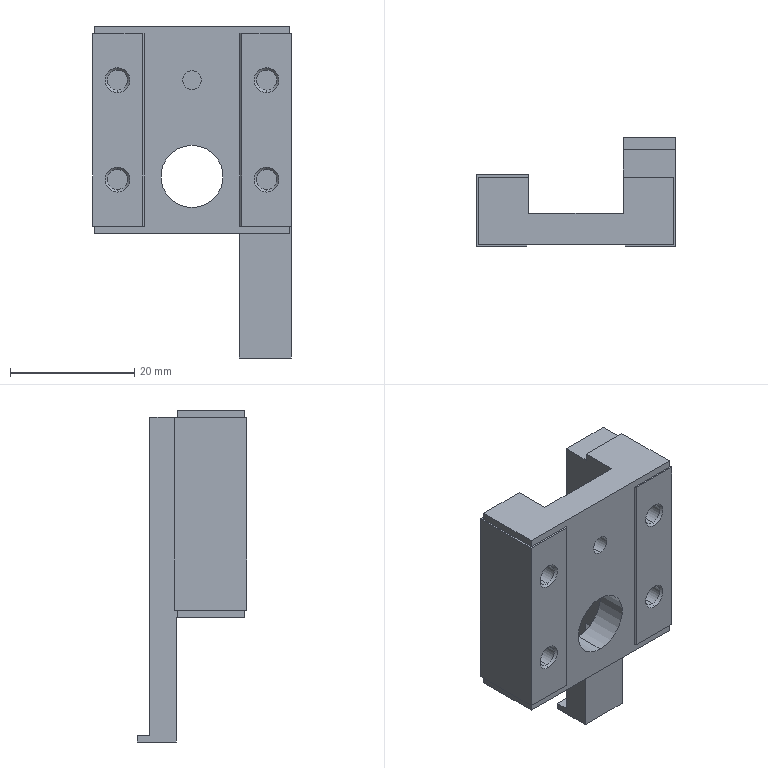Part | SolidWorks | features BaseBody 1 | 1 solid | 54 faces | box 32 x 17.6 x 53.4 mm | volume 10272 mm3 | plane 34 | cylinder 12 | cone 8 | commonest cylinder face diameters 3.242 x8 3 x2 10 x2
STEP:
#1=CARTESIAN_POINT('',(12.,0.379,7.079));
#2=VERTEX_POINT('',#1);
#3=CARTESIAN_POINT('',(12.,0.379,10.321));
#4=VERTEX_POINT('',#3);
#5=CARTESIAN_POINT('',(12.,0.379,8.7));
#6=DIRECTION('',(0.,-1.,0.));
#7=DIRECTION('',(0.,0.,-1.));
#8=AXIS2_PLACEMENT_3D('',#5,#6,#7);
#9=CIRCLE('',#8,1.621);
#10=EDGE_CURVE('',#2,#4,#9,.T.);
#11=ORIENTED_EDGE('',*,*,#10,.T.);
#12=CARTESIAN_POINT('',(12.,4.,10.321));
#13=VERTEX_POINT('',#12);
#14=CARTESIAN_POINT('',(12.,0.,10.321));
#15=DIRECTION('',(0.,1.,0.));
#16=VECTOR('',#15,1000.);
#17=LINE('',#14,#16);
#18=EDGE_CURVE('',#4,#13,#17,.T.);
#19=ORIENTED_EDGE('',*,*,#18,.T.);
#20=CARTESIAN_POINT('',(12.,4.,7.079));
#21=VERTEX_POINT('',#20);
#22=CARTESIAN_POINT('',(12.,4.,8.7));
#23=DIRECTION('',(0.,-1.,0.));
#24=DIRECTION('',(0.,0.,-1.));
#25=AXIS2_PLACEMENT_3D('',#22,#23,#24);
#26=CIRCLE('',#25,1.621);
#27=EDGE_CURVE('',#21,#13,#26,.T.);
#28=ORIENTED_EDGE('',*,*,#27,.F.);
#29=CARTESIAN_POINT('',(12.,0.,7.079));
#30=DIRECTION('',(0.,1.,0.));
#31=VECTOR('',#30,1000.);
#32=LINE('',#29,#31);
#33=EDGE_CURVE('',#2,#21,#32,.T.);
#34=ORIENTED_EDGE('',*,*,#33,.F.);
#35=EDGE_LOOP('',(#11,#19,#28,#34));
#36=FACE_OUTER_BOUND('',#35,.T.);
#37=CARTESIAN_POINT('',(12.,0.,8.7));
#38=DIRECTION('',(0.,1.,0.));
#39=DIRECTION('',(0.,0.,-1.));
#40=AXIS2_PLACEMENT_3D('',#37,#38,#39);
#41=CYLINDRICAL_SURFACE('',#40,1.621);
#42=ADVANCED_FACE('',(#36),#41,.F.);
#43=CARTESIAN_POINT('',(12.,0.379,8.7));
#44=DIRECTION('',(0.,-1.,0.));
#45=DIRECTION('',(0.,0.,-1.));
#46=AXIS2_PLACEMENT_3D('',#43,#44,#45);
#47=CIRCLE('',#46,1.621);
#48=EDGE_CURVE('',#4,#2,#47,.T.);
#49=ORIENTED_EDGE('',*,*,#48,.F.);
#50=CARTESIAN_POINT('',(12.,0.,10.7));
#51=VERTEX_POINT('',#50);
#52=CARTESIAN_POINT('',(12.,0.379,10.321));
#53=DIRECTION('',(0.,-0.7071,0.7071));
#54=VECTOR('',#53,1000.);
#55=LINE('',#52,#54);
#56=EDGE_CURVE('',#4,#51,#55,.T.);
#57=ORIENTED_EDGE('',*,*,#56,.T.);
#58=CARTESIAN_POINT('',(12.,0.,6.7));
#59=VERTEX_POINT('',#58);
#60=CARTESIAN_POINT('',(12.,0.,8.7));
#61=DIRECTION('',(0.,-1.,0.));
#62=DIRECTION('',(0.,0.,-1.));
#63=AXIS2_PLACEMENT_3D('',#60,#61,#62);
#64=CIRCLE('',#63,2.);
#65=EDGE_CURVE('',#51,#59,#64,.T.);
#66=ORIENTED_EDGE('',*,*,#65,.T.);
#67=CARTESIAN_POINT('',(12.,0.379,7.079));
#68=DIRECTION('',(0.,-0.7071,-0.7071));
#69=VECTOR('',#68,1000.);
#70=LINE('',#67,#69);
#71=EDGE_CURVE('',#2,#59,#70,.T.);
#72=ORIENTED_EDGE('',*,*,#71,.F.);
#73=EDGE_LOOP('',(#49,#57,#66,#72));
#74=FACE_OUTER_BOUND('',#73,.T.);
#75=CARTESIAN_POINT('',(12.,0.379,8.7));
#76=DIRECTION('',(0.,-1.,0.));
#77=DIRECTION('',(0.,0.,-1.));
#78=AXIS2_PLACEMENT_3D('',#75,#76,#77);
#79=CONICAL_SURFACE('',#78,1.621,0.7854);
#80=ADVANCED_FACE('',(#74),#79,.F.);
#81=CARTESIAN_POINT('',(-12.,0.379,7.079));
#82=VERTEX_POINT('',#81);
#83=CARTESIAN_POINT('',(-12.,0.379,10.321));
#84=VERTEX_POINT('',#83);
#85=CARTESIAN_POINT('',(-12.,0.379,8.7));
#86=DIRECTION('',(0.,-1.,0.));
#87=DIRECTION('',(0.,0.,-1.));
#88=AXIS2_PLACEMENT_3D('',#85,#86,#87);
#89=CIRCLE('',#88,1.621);
#90=EDGE_CURVE('',#82,#84,#89,.T.);
#91=ORIENTED_EDGE('',*,*,#90,.T.);
#92=CARTESIAN_POINT('',(-12.,4.,10.321));
#93=VERTEX_POINT('',#92);
#94=CARTESIAN_POINT('',(-12.,0.,10.321));
#95=DIRECTION('',(0.,1.,0.));
#96=VECTOR('',#95,1000.);
#97=LINE('',#94,#96);
#98=EDGE_CURVE('',#84,#93,#97,.T.);
#99=ORIENTED_EDGE('',*,*,#98,.T.);
#100=CARTESIAN_POINT('',(-12.,4.,7.079));
#101=VERTEX_POINT('',#100);
#102=CARTESIAN_POINT('',(-12.,4.,8.7));
#103=DIRECTION('',(0.,-1.,0.));
#104=DIRECTION('',(0.,0.,-1.));
#105=AXIS2_PLACEMENT_3D('',#102,#103,#104);
#106=CIRCLE('',#105,1.621);
#107=EDGE_CURVE('',#101,#93,#106,.T.);
#108=ORIENTED_EDGE('',*,*,#107,.F.);
#109=CARTESIAN_POINT('',(-12.,0.,7.079));
#110=DIRECTION('',(0.,1.,0.));
#111=VECTOR('',#110,1000.);
#112=LINE('',#109,#111);
#113=EDGE_CURVE('',#82,#101,#112,.T.);
#114=ORIENTED_EDGE('',*,*,#113,.F.);
#115=EDGE_LOOP('',(#91,#99,#108,#114));
#116=FACE_OUTER_BOUND('',#115,.T.);
#117=CARTESIAN_POINT('',(-12.,0.,8.7));
#118=DIRECTION('',(0.,1.,0.));
#119=DIRECTION('',(0.,0.,-1.));
#120=AXIS2_PLACEMENT_3D('',#117,#118,#119);
#121=CYLINDRICAL_SURFACE('',#120,1.621);
#122=ADVANCED_FACE('',(#116),#121,.F.);
#123=CARTESIAN_POINT('',(-12.,0.379,8.7));
#124=DIRECTION('',(0.,-1.,0.));
#125=DIRECTION('',(0.,0.,-1.));
#126=AXIS2_PLACEMENT_3D('',#123,#124,#125);
#127=CIRCLE('',#126,1.621);
#128=EDGE_CURVE('',#84,#82,#127,.T.);
#129=ORIENTED_EDGE('',*,*,#128,.F.);
#130=CARTESIAN_POINT('',(-12.,0.,10.7));
#131=VERTEX_POINT('',#130);
#132=CARTESIAN_POINT('',(-12.,0.379,10.321));
#133=DIRECTION('',(0.,-0.7071,0.7071));
#134=VECTOR('',#133,1000.);
#135=LINE('',#132,#134);
#136=EDGE_CURVE('',#84,#131,#135,.T.);
#137=ORIENTED_EDGE('',*,*,#136,.T.);
#138=CARTESIAN_POINT('',(-12.,0.,6.7));
#139=VERTEX_POINT('',#138);
#140=CARTESIAN_POINT('',(-12.,0.,8.7));
#141=DIRECTION('',(0.,-1.,0.));
#142=DIRECTION('',(0.,0.,-1.));
#143=AXIS2_PLACEMENT_3D('',#140,#141,#142);
#144=CIRCLE('',#143,2.);
#145=EDGE_CURVE('',#131,#139,#144,.T.);
#146=ORIENTED_EDGE('',*,*,#145,.T.);
#147=CARTESIAN_POINT('',(-12.,0.379,7.079));
#148=DIRECTION('',(0.,-0.7071,-0.7071));
#149=VECTOR('',#148,1000.);
#150=LINE('',#147,#149);
#151=EDGE_CURVE('',#82,#139,#150,.T.);
#152=ORIENTED_EDGE('',*,*,#151,.F.);
#153=EDGE_LOOP('',(#129,#137,#146,#152));
#154=FACE_OUTER_BOUND('',#153,.T.);
#155=CARTESIAN_POINT('',(-12.,0.379,8.7));
#156=DIRECTION('',(0.,-1.,0.));
#157=DIRECTION('',(0.,0.,-1.));
#158=AXIS2_PLACEMENT_3D('',#155,#156,#157);
#159=CONICAL_SURFACE('',#158,1.621,0.7854);
#160=ADVANCED_FACE('',(#154),#159,.F.);
#161=CARTESIAN_POINT('',(12.,0.379,23.079));
#162=VERTEX_POINT('',#161);
#163=CARTESIAN_POINT('',(12.,0.379,26.321));
#164=VERTEX_POINT('',#163);
#165=CARTESIAN_POINT('',(12.,0.379,24.7));
#166=DIRECTION('',(0.,-1.,0.));
#167=DIRECTION('',(0.,0.,-1.));
#168=AXIS2_PLACEMENT_3D('',#165,#166,#167);
#169=CIRCLE('',#168,1.621);
#170=EDGE_CURVE('',#162,#164,#169,.T.);
#171=ORIENTED_EDGE('',*,*,#170,.T.);
#172=CARTESIAN_POINT('',(12.,4.,26.321));
#173=VERTEX_POINT('',#172);
#174=CARTESIAN_POINT('',(12.,0.,26.321));
#175=DIRECTION('',(0.,1.,0.));
#176=VECTOR('',#175,1000.);
#177=LINE('',#174,#176);
#178=EDGE_CURVE('',#164,#173,#177,.T.);
#179=ORIENTED_EDGE('',*,*,#178,.T.);
#180=CARTESIAN_POINT('',(12.,4.,23.079));
#181=VERTEX_POINT('',#180);
#182=CARTESIAN_POINT('',(12.,4.,24.7));
#183=DIRECTION('',(0.,-1.,0.));
#184=DIRECTION('',(0.,0.,-1.));
#185=AXIS2_PLACEMENT_3D('',#182,#183,#184);
#186=CIRCLE('',#185,1.621);
#187=EDGE_CURVE('',#181,#173,#186,.T.);
#188=ORIENTED_EDGE('',*,*,#187,.F.);
#189=CARTESIAN_POINT('',(12.,0.,23.079));
#190=DIRECTION('',(0.,1.,0.));
#191=VECTOR('',#190,1000.);
#192=LINE('',#189,#191);
#193=EDGE_CURVE('',#162,#181,#192,.T.);
#194=ORIENTED_EDGE('',*,*,#193,.F.);
#195=EDGE_LOOP('',(#171,#179,#188,#194));
#196=FACE_OUTER_BOUND('',#195,.T.);
#197=CARTESIAN_POINT('',(12.,0.,24.7));
#198=DIRECTION('',(0.,1.,0.));
#199=DIRECTION('',(0.,0.,-1.));
#200=AXIS2_PLACEMENT_3D('',#197,#198,#199);
#201=CYLINDRICAL_SURFACE('',#200,1.621);
#202=ADVANCED_FACE('',(#196),#201,.F.);
#203=CARTESIAN_POINT('',(12.,0.379,24.7));
#204=DIRECTION('',(0.,-1.,0.));
#205=DIRECTION('',(0.,0.,-1.));
#206=AXIS2_PLACEMENT_3D('',#203,#204,#205);
#207=CIRCLE('',#206,1.621);
#208=EDGE_CURVE('',#164,#162,#207,.T.);
#209=ORIENTED_EDGE('',*,*,#208,.F.);
#210=CARTESIAN_POINT('',(12.,0.,26.7));
#211=VERTEX_POINT('',#210);
#212=CARTESIAN_POINT('',(12.,0.379,26.321));
#213=DIRECTION('',(0.,-0.7071,0.7071));
#214=VECTOR('',#213,1000.);
#215=LINE('',#212,#214);
#216=EDGE_CURVE('',#164,#211,#215,.T.);
#217=ORIENTED_EDGE('',*,*,#216,.T.);
#218=CARTESIAN_POINT('',(12.,0.,22.7));
#219=VERTEX_POINT('',#218);
#220=CARTESIAN_POINT('',(12.,0.,24.7));
#221=DIRECTION('',(0.,-1.,0.));
#222=DIRECTION('',(0.,0.,-1.));
#223=AXIS2_PLACEMENT_3D('',#220,#221,#222);
#224=CIRCLE('',#223,2.);
#225=EDGE_CURVE('',#211,#219,#224,.T.);
#226=ORIENTED_EDGE('',*,*,#225,.T.);
#227=CARTESIAN_POINT('',(12.,0.379,23.079));
#228=DIRECTION('',(0.,-0.7071,-0.7071));
#229=VECTOR('',#228,1000.);
#230=LINE('',#227,#229);
#231=EDGE_CURVE('',#162,#219,#230,.T.);
#232=ORIENTED_EDGE('',*,*,#231,.F.);
#233=EDGE_LOOP('',(#209,#217,#226,#232));
#234=FACE_OUTER_BOUND('',#233,.T.);
#235=CARTESIAN_POINT('',(12.,0.379,24.7));
#236=DIRECTION('',(0.,-1.,0.));
#237=DIRECTION('',(0.,0.,-1.));
#238=AXIS2_PLACEMENT_3D('',#235,#236,#237);
#239=CONICAL_SURFACE('',#238,1.621,0.7854);
#240=ADVANCED_FACE('',(#234),#239,.F.);
#241=CARTESIAN_POINT('',(-12.,0.379,23.079));
#242=VERTEX_POINT('',#241);
#243=CARTESIAN_POINT('',(-12.,0.379,26.321));
#244=VERTEX_POINT('',#243);
#245=CARTESIAN_POINT('',(-12.,0.379,24.7));
#246=DIRECTION('',(0.,-1.,0.));
#247=DIRECTION('',(0.,0.,-1.));
#248=AXIS2_PLACEMENT_3D('',#245,#246,#247);
#249=CIRCLE('',#248,1.621);
#250=EDGE_CURVE('',#242,#244,#249,.T.);
#251=ORIENTED_EDGE('',*,*,#250,.T.);
#252=CARTESIAN_POINT('',(-12.,4.,26.321));
#253=VERTEX_POINT('',#252);
#254=CARTESIAN_POINT('',(-12.,0.,26.321));
#255=DIRECTION('',(0.,1.,0.));
#256=VECTOR('',#255,1000.);
#257=LINE('',#254,#256);
#258=EDGE_CURVE('',#244,#253,#257,.T.);
#259=ORIENTED_EDGE('',*,*,#258,.T.);
#260=CARTESIAN_POINT('',(-12.,4.,23.079));
#261=VERTEX_POINT('',#260);
#262=CARTESIAN_POINT('',(-12.,4.,24.7));
#263=DIRECTION('',(0.,-1.,0.));
#264=DIRECTION('',(0.,0.,-1.));
#265=AXIS2_PLACEMENT_3D('',#262,#263,#264);
#266=CIRCLE('',#265,1.621);
#267=EDGE_CURVE('',#261,#253,#266,.T.);
#268=ORIENTED_EDGE('',*,*,#267,.F.);
#269=CARTESIAN_POINT('',(-12.,0.,23.079));
#270=DIRECTION('',(0.,1.,0.));
#271=VECTOR('',#270,1000.);
#272=LINE('',#269,#271);
#273=EDGE_CURVE('',#242,#261,#272,.T.);
#274=ORIENTED_EDGE('',*,*,#273,.F.);
#275=EDGE_LOOP('',(#251,#259,#268,#274));
#276=FACE_OUTER_BOUND('',#275,.T.);
#277=CARTESIAN_POINT('',(-12.,0.,24.7));
#278=DIRECTION('',(0.,1.,0.));
#279=DIRECTION('',(0.,0.,-1.));
#280=AXIS2_PLACEMENT_3D('',#277,#278,#279);
#281=CYLINDRICAL_SURFACE('',#280,1.621);
#282=ADVANCED_FACE('',(#276),#281,.F.);
#283=CARTESIAN_POINT('',(-12.,0.379,24.7));
#284=DIRECTION('',(0.,-1.,0.));
#285=DIRECTION('',(0.,0.,-1.));
#286=AXIS2_PLACEMENT_3D('',#283,#284,#285);
#287=CIRCLE('',#286,1.621);
#288=EDGE_CURVE('',#244,#242,#287,.T.);
#289=ORIENTED_EDGE('',*,*,#288,.F.);
#290=CARTESIAN_POINT('',(-12.,0.,26.7));
#291=VERTEX_POINT('',#290);
#292=CARTESIAN_POINT('',(-12.,0.379,26.321));
#293=DIRECTION('',(0.,-0.7071,0.7071));
#294=VECTOR('',#293,1000.);
#295=LINE('',#292,#294);
#296=EDGE_CURVE('',#244,#291,#295,.T.);
#297=ORIENTED_EDGE('',*,*,#296,.T.);
#298=CARTESIAN_POINT('',(-12.,0.,22.7));
#299=VERTEX_POINT('',#298);
#300=CARTESIAN_POINT('',(-12.,0.,24.7));
#301=DIRECTION('',(0.,-1.,0.));
#302=DIRECTION('',(0.,0.,-1.));
#303=AXIS2_PLACEMENT_3D('',#300,#301,#302);
#304=CIRCLE('',#303,2.);
#305=EDGE_CURVE('',#291,#299,#304,.T.);
#306=ORIENTED_EDGE('',*,*,#305,.T.);
#307=CARTESIAN_POINT('',(-12.,0.379,23.079));
#308=DIRECTION('',(0.,-0.7071,-0.7071));
#309=VECTOR('',#308,1000.);
#310=LINE('',#307,#309);
#311=EDGE_CURVE('',#242,#299,#310,.T.);
#312=ORIENTED_EDGE('',*,*,#311,.F.);
#313=EDGE_LOOP('',(#289,#297,#306,#312));
#314=FACE_OUTER_BOUND('',#313,.T.);
#315=CARTESIAN_POINT('',(-12.,0.379,24.7));
#316=DIRECTION('',(0.,-1.,0.));
#317=DIRECTION('',(0.,0.,-1.));
#318=AXIS2_PLACEMENT_3D('',#315,#316,#317);
#319=CONICAL_SURFACE('',#318,1.621,0.7854);
#320=ADVANCED_FACE('',(#314),#319,.F.);
#321=CARTESIAN_POINT('',(0.,0.3,23.2));
#322=VERTEX_POINT('',#321);
#323=CARTESIAN_POINT('',(0.,0.3,26.2));
#324=VERTEX_POINT('',#323);
#325=CARTESIAN_POINT('',(0.,0.3,24.7));
#326=DIRECTION('',(0.,-1.,0.));
#327=DIRECTION('',(0.,0.,1.));
#328=AXIS2_PLACEMENT_3D('',#325,#326,#327);
#329=CIRCLE('',#328,1.5);
#330=EDGE_CURVE('',#322,#324,#329,.T.);
#331=ORIENTED_EDGE('',*,*,#330,.T.);
#332=CARTESIAN_POINT('',(0.,3.3,26.2));
#333=VERTEX_POINT('',#332);
#334=CARTESIAN_POINT('',(0.,3.3,26.2));
#335=DIRECTION('',(0.,1.,0.));
#336=VECTOR('',#335,1000.);
#337=LINE('',#334,#336);
#338=EDGE_CURVE('',#324,#333,#337,.T.);
#339=ORIENTED_EDGE('',*,*,#338,.T.);
#340=CARTESIAN_POINT('',(0.,3.3,23.2));
#341=VERTEX_POINT('',#340);
#342=CARTESIAN_POINT('',(0.,3.3,24.7));
#343=DIRECTION('',(0.,1.,0.));
#344=DIRECTION('',(1.,0.,0.));
#345=AXIS2_PLACEMENT_3D('',#342,#343,#344);
#346=CIRCLE('',#345,1.5);
#347=EDGE_CURVE('',#333,#341,#346,.T.);
#348=ORIENTED_EDGE('',*,*,#347,.T.);
#349=CARTESIAN_POINT('',(0.,3.3,23.2));
#350=DIRECTION('',(0.,1.,0.));
#351=VECTOR('',#350,1000.);
#352=LINE('',#349,#351);
#353=EDGE_CURVE('',#322,#341,#352,.T.);
#354=ORIENTED_EDGE('',*,*,#353,.F.);
#355=EDGE_LOOP('',(#331,#339,#348,#354));
#356=FACE_OUTER_BOUND('',#355,.T.);
#357=CARTESIAN_POINT('',(0.,3.3,24.7));
#358=DIRECTION('',(0.,1.,0.));
#359=DIRECTION('',(0.,0.,-1.));
#360=AXIS2_PLACEMENT_3D('',#357,#358,#359);
#361=CYLINDRICAL_SURFACE('',#360,1.5);
#362=ADVANCED_FACE('',(#356),#361,.F.);
#363=CARTESIAN_POINT('',(0.,0.3,4.2));
#364=VERTEX_POINT('',#363);
#365=CARTESIAN_POINT('',(0.,0.3,14.2));
#366=VERTEX_POINT('',#365);
#367=CARTESIAN_POINT('',(0.,0.3,9.2));
#368=DIRECTION('',(0.,-1.,0.));
#369=DIRECTION('',(0.,0.,1.));
#370=AXIS2_PLACEMENT_3D('',#367,#368,#369);
#371=CIRCLE('',#370,5.);
#372=EDGE_CURVE('',#364,#366,#371,.T.);
#373=ORIENTED_EDGE('',*,*,#372,.T.);
#374=CARTESIAN_POINT('',(0.,5.3,14.2));
#375=VERTEX_POINT('',#374);
#376=CARTESIAN_POINT('',(0.,5.5,14.2));
#377=DIRECTION('',(0.,1.,0.));
#378=VECTOR('',#377,1000.);
#379=LINE('',#376,#378);
#380=EDGE_CURVE('',#366,#375,#379,.T.);
#381=ORIENTED_EDGE('',*,*,#380,.T.);
#382=CARTESIAN_POINT('',(0.,5.3,4.2));
#383=VERTEX_POINT('',#382);
#384=CARTESIAN_POINT('',(0.,5.3,9.2));
#385=DIRECTION('',(0.,1.,0.));
#386=DIRECTION('',(0.,0.,-1.));
#387=AXIS2_PLACEMENT_3D('',#384,#385,#386);
#388=CIRCLE('',#387,5.);
#389=EDGE_CURVE('',#375,#383,#388,.T.);
#390=ORIENTED_EDGE('',*,*,#389,.T.);
#391=CARTESIAN_POINT('',(0.,5.5,4.2));
#392=DIRECTION('',(0.,1.,0.));
#393=VECTOR('',#392,1000.);
#394=LINE('',#391,#393);
#395=EDGE_CURVE('',#364,#383,#394,.T.);
#396=ORIENTED_EDGE('',*,*,#395,.F.);
#397=EDGE_LOOP('',(#373,#381,#390,#396));
#398=FACE_OUTER_BOUND('',#397,.T.);
#399=CARTESIAN_POINT('',(0.,5.5,9.2));
#400=DIRECTION('',(0.,1.,0.));
#401=DIRECTION('',(0.,0.,-1.));
#402=AXIS2_PLACEMENT_3D('',#399,#400,#401);
#403=CYLINDRICAL_SURFACE('',#402,5.);
#404=ADVANCED_FACE('',(#398),#403,.F.);
#405=CARTESIAN_POINT('',(15.7,11.3,1.2));
#406=VERTEX_POINT('',#405);
#407=CARTESIAN_POINT('',(15.7,0.3,1.2));
#408=VERTEX_POINT('',#407);
#409=CARTESIAN_POINT('',(15.7,11.6,1.2));
#410=DIRECTION('',(0.,-1.,0.));
#411=VECTOR('',#410,1000.);
#412=LINE('',#409,#411);
#413=EDGE_CURVE('',#406,#408,#412,.T.);
#414=ORIENTED_EDGE('',*,*,#413,.F.);
#415=CARTESIAN_POINT('',(16.,11.3,1.2));
#416=VERTEX_POINT('',#415);
#417=CARTESIAN_POINT('',(7.6,11.3,1.2));
#418=DIRECTION('',(1.,0.,0.));
#419=VECTOR('',#418,1000.);
#420=LINE('',#417,#419);
#421=EDGE_CURVE('',#406,#416,#420,.T.);
#422=ORIENTED_EDGE('',*,*,#421,.T.);
#423=CARTESIAN_POINT('',(16.,0.,1.2));
#424=VERTEX_POINT('',#423);
#425=CARTESIAN_POINT('',(16.,0.,1.2));
#426=DIRECTION('',(0.,1.,0.));
#427=VECTOR('',#426,1000.);
#428=LINE('',#425,#427);
#429=EDGE_CURVE('',#424,#416,#428,.T.);
#430=ORIENTED_EDGE('',*,*,#429,.F.);
#431=CARTESIAN_POINT('',(8.,0.,1.2));
#432=VERTEX_POINT('',#431);
#433=CARTESIAN_POINT('',(-16.,0.,1.2));
#434=DIRECTION('',(1.,0.,0.));
#435=VECTOR('',#434,1000.);
#436=LINE('',#433,#435);
#437=EDGE_CURVE('',#432,#424,#436,.T.);
#438=ORIENTED_EDGE('',*,*,#437,.F.);
#439=CARTESIAN_POINT('',(7.7,0.3,1.2));
#440=VERTEX_POINT('',#439);
#441=CARTESIAN_POINT('',(7.7,0.3,1.2));
#442=DIRECTION('',(0.7071,-0.7071,0.));
#443=VECTOR('',#442,1000.);
#444=LINE('',#441,#443);
#445=EDGE_CURVE('',#440,#432,#444,.T.);
#446=ORIENTED_EDGE('',*,*,#445,.F.);
#447=CARTESIAN_POINT('',(15.7,0.3,1.2));
#448=DIRECTION('',(-1.,0.,0.));
#449=VECTOR('',#448,1000.);
#450=LINE('',#447,#449);
#451=EDGE_CURVE('',#408,#440,#450,.T.);
#452=ORIENTED_EDGE('',*,*,#451,.F.);
#453=EDGE_LOOP('',(#414,#422,#430,#438,#446,#452));
#454=FACE_OUTER_BOUND('',#453,.T.);
#455=CARTESIAN_POINT('',(0.,0.,1.2));
#456=DIRECTION('',(0.,0.,1.));
#457=DIRECTION('',(1.,0.,0.));
#458=AXIS2_PLACEMENT_3D('',#455,#456,#457);
#459=PLANE('',#458);
#460=ADVANCED_FACE('',(#454),#459,.F.);
#461=CARTESIAN_POINT('',(7.7,0.3,32.2));
#462=VERTEX_POINT('',#461);
#463=CARTESIAN_POINT('',(8.,0.,32.2));
#464=VERTEX_POINT('',#463);
#465=CARTESIAN_POINT('',(7.7,0.3,32.2));
#466=DIRECTION('',(0.7071,-0.7071,0.));
#467=VECTOR('',#466,1000.);
#468=LINE('',#465,#467);
#469=EDGE_CURVE('',#462,#464,#468,.T.);
#470=ORIENTED_EDGE('',*,*,#469,.T.);
#471=CARTESIAN_POINT('',(16.,0.,32.2));
#472=VERTEX_POINT('',#471);
#473=CARTESIAN_POINT('',(-16.,0.,32.2));
#474=DIRECTION('',(1.,0.,0.));
#475=VECTOR('',#474,1000.);
#476=LINE('',#473,#475);
#477=EDGE_CURVE('',#464,#472,#476,.T.);
#478=ORIENTED_EDGE('',*,*,#477,.T.);
#479=CARTESIAN_POINT('',(16.,15.6,32.2));
#480=VERTEX_POINT('',#479);
#481=CARTESIAN_POINT('',(16.,0.,32.2));
#482=DIRECTION('',(0.,1.,0.));
#483=VECTOR('',#482,1000.);
#484=LINE('',#481,#483);
#485=EDGE_CURVE('',#472,#480,#484,.T.);
#486=ORIENTED_EDGE('',*,*,#485,.T.);
#487=CARTESIAN_POINT('',(7.6,15.6,32.2));
#488=VERTEX_POINT('',#487);
#489=CARTESIAN_POINT('',(16.,15.6,32.2));
#490=DIRECTION('',(-1.,0.,0.));
#491=VECTOR('',#490,1000.);
#492=LINE('',#489,#491);
#493=EDGE_CURVE('',#480,#488,#492,.T.);
#494=ORIENTED_EDGE('',*,*,#493,.T.);
#495=CARTESIAN_POINT('',(7.6,11.1,32.2));
#496=VERTEX_POINT('',#495);
#497=CARTESIAN_POINT('',(7.6,15.6,32.2));
#498=DIRECTION('',(0.,-1.,0.));
#499=VECTOR('',#498,1000.);
#500=LINE('',#497,#499);
#501=EDGE_CURVE('',#488,#496,#500,.T.);
#502=ORIENTED_EDGE('',*,*,#501,.T.);
#503=CARTESIAN_POINT('',(15.7,11.1,32.2));
#504=VERTEX_POINT('',#503);
#505=CARTESIAN_POINT('',(7.6,11.1,32.2));
#506=DIRECTION('',(1.,0.,0.));
#507=VECTOR('',#506,1000.);
#508=LINE('',#505,#507);
#509=EDGE_CURVE('',#496,#504,#508,.T.);
#510=ORIENTED_EDGE('',*,*,#509,.T.);
#511=CARTESIAN_POINT('',(15.7,0.3,32.2));
#512=VERTEX_POINT('',#511);
#513=CARTESIAN_POINT('',(15.7,11.1,32.2));
#514=DIRECTION('',(0.,-1.,0.));
#515=VECTOR('',#514,1000.);
#516=LINE('',#513,#515);
#517=EDGE_CURVE('',#504,#512,#516,.T.);
#518=ORIENTED_EDGE('',*,*,#517,.T.);
#519=CARTESIAN_POINT('',(15.7,0.3,32.2));
#520=DIRECTION('',(-1.,0.,0.));
#521=VECTOR('',#520,1000.);
#522=LINE('',#519,#521);
#523=EDGE_CURVE('',#512,#462,#522,.T.);
#524=ORIENTED_EDGE('',*,*,#523,.T.);
#525=EDGE_LOOP('',(#470,#478,#486,#494,#502,#510,#518,#524));
#526=FACE_OUTER_BOUND('',#525,.T.);
#527=CARTESIAN_POINT('',(0.,0.,32.2));
#528=DIRECTION('',(0.,0.,1.));
#529=DIRECTION('',(1.,0.,0.));
#530=AXIS2_PLACEMENT_3D('',#527,#528,#529);
#531=PLANE('',#530);
#532=ADVANCED_FACE('',(#526),#531,.T.);
#533=CARTESIAN_POINT('',(16.,17.6,-19.));
#534=VERTEX_POINT('',#533);
#535=CARTESIAN_POINT('',(7.6,17.6,-19.));
#536=VERTEX_POINT('',#535);
#537=CARTESIAN_POINT('',(16.,17.6,-19.));
#538=DIRECTION('',(-1.,0.,0.));
#539=VECTOR('',#538,1000.);
#540=LINE('',#537,#539);
#541=EDGE_CURVE('',#534,#536,#540,.T.);
#542=ORIENTED_EDGE('',*,*,#541,.T.);
#543=CARTESIAN_POINT('',(7.6,15.6,-19.));
#544=VERTEX_POINT('',#543);
#545=CARTESIAN_POINT('',(7.6,17.6,-19.));
#546=DIRECTION('',(0.,-1.,0.));
#547=VECTOR('',#546,1000.);
#548=LINE('',#545,#547);
#549=EDGE_CURVE('',#536,#544,#548,.T.);
#550=ORIENTED_EDGE('',*,*,#549,.T.);
#551=CARTESIAN_POINT('',(16.,15.6,-19.));
#552=VERTEX_POINT('',#551);
#553=CARTESIAN_POINT('',(7.6,15.6,-19.));
#554=DIRECTION('',(1.,0.,0.));
#555=VECTOR('',#554,1000.);
#556=LINE('',#553,#555);
#557=EDGE_CURVE('',#544,#552,#556,.T.);
#558=ORIENTED_EDGE('',*,*,#557,.T.);
#559=CARTESIAN_POINT('',(16.,15.6,-19.));
#560=DIRECTION('',(0.,1.,0.));
#561=VECTOR('',#560,1000.);
#562=LINE('',#559,#561);
#563=EDGE_CURVE('',#552,#534,#562,.T.);
#564=ORIENTED_EDGE('',*,*,#563,.T.);
#565=EDGE_LOOP('',(#542,#550,#558,#564));
#566=FACE_OUTER_BOUND('',#565,.T.);
#567=CARTESIAN_POINT('',(0.,0.,-19.));
#568=DIRECTION('',(0.,0.,1.));
#569=DIRECTION('',(1.,0.,0.));
#570=AXIS2_PLACEMENT_3D('',#567,#568,#569);
#571=PLANE('',#570);
#572=ADVANCED_FACE('',(#566),#571,.T.);
#573=CARTESIAN_POINT('',(16.,17.6,-20.));
#574=VERTEX_POINT('',#573);
#575=CARTESIAN_POINT('',(7.6,17.6,-20.));
#576=VERTEX_POINT('',#575);
#577=CARTESIAN_POINT('',(16.,17.6,-20.));
#578=DIRECTION('',(-1.,0.,0.));
#579=VECTOR('',#578,1000.);
#580=LINE('',#577,#579);
#581=EDGE_CURVE('',#574,#576,#580,.T.);
#582=ORIENTED_EDGE('',*,*,#581,.T.);
#583=CARTESIAN_POINT('',(7.6,17.6,-19.));
#584=DIRECTION('',(0.,0.,-1.));
#585=VECTOR('',#584,1000.);
#586=LINE('',#583,#585);
#587=EDGE_CURVE('',#536,#576,#586,.T.);
#588=ORIENTED_EDGE('',*,*,#587,.F.);
#589=ORIENTED_EDGE('',*,*,#541,.F.);
#590=CARTESIAN_POINT('',(16.,17.6,-19.));
#591=DIRECTION('',(0.,0.,-1.));
#592=VECTOR('',#591,1000.);
#593=LINE('',#590,#592);
#594=EDGE_CURVE('',#534,#574,#593,.T.);
#595=ORIENTED_EDGE('',*,*,#594,.T.);
#596=EDGE_LOOP('',(#582,#588,#589,#595));
#597=FACE_OUTER_BOUND('',#596,.T.);
#598=CARTESIAN_POINT('',(16.,17.6,-19.));
#599=DIRECTION('',(0.,-1.,0.));
#600=DIRECTION('',(0.,0.,-1.));
#601=AXIS2_PLACEMENT_3D('',#598,#599,#600);
#602=PLANE('',#601);
#603=ADVANCED_FACE('',(#597),#602,.F.);
#604=ORIENTED_EDGE('',*,*,#380,.F.);
#605=CARTESIAN_POINT('',(0.,0.3,9.2));
#606=DIRECTION('',(0.,-1.,0.));
#607=DIRECTION('',(0.,0.,1.));
#608=AXIS2_PLACEMENT_3D('',#605,#606,#607);
#609=CIRCLE('',#608,5.);
#610=EDGE_CURVE('',#366,#364,#609,.T.);
#611=ORIENTED_EDGE('',*,*,#610,.T.);
#612=ORIENTED_EDGE('',*,*,#395,.T.);
#613=CARTESIAN_POINT('',(0.,5.3,9.2));
#614=DIRECTION('',(0.,1.,0.));
#615=DIRECTION('',(0.,0.,-1.));
#616=AXIS2_PLACEMENT_3D('',#613,#614,#615);
#617=CIRCLE('',#616,5.);
#618=EDGE_CURVE('',#383,#375,#617,.T.);
#619=ORIENTED_EDGE('',*,*,#618,.T.);
#620=EDGE_LOOP('',(#604,#611,#612,#619));
#621=FACE_OUTER_BOUND('',#620,.T.);
#622=CARTESIAN_POINT('',(0.,5.5,9.2));
#623=DIRECTION('',(0.,1.,0.));
#624=DIRECTION('',(0.,0.,-1.));
#625=AXIS2_PLACEMENT_3D('',#622,#623,#624);
#626=CYLINDRICAL_SURFACE('',#625,5.);
#627=ADVANCED_FACE('',(#621),#626,.F.);
#628=CARTESIAN_POINT('',(0.,3.3,24.7));
#629=DIRECTION('',(0.,1.,0.));
#630=DIRECTION('',(1.,0.,0.));
#631=AXIS2_PLACEMENT_3D('',#628,#629,#630);
#632=CIRCLE('',#631,1.5);
#633=EDGE_CURVE('',#341,#333,#632,.T.);
#634=ORIENTED_EDGE('',*,*,#633,.F.);
#635=ORIENTED_EDGE('',*,*,#347,.F.);
#636=EDGE_LOOP('',(#634,#635));
#637=FACE_OUTER_BOUND('',#636,.T.);
#638=CARTESIAN_POINT('',(0.,3.3,24.7));
#639=DIRECTION('',(0.,1.,0.));
#640=DIRECTION('',(1.,0.,0.));
#641=AXIS2_PLACEMENT_3D('',#638,#639,#640);
#642=PLANE('',#641);
#643=ADVANCED_FACE('',(#637),#642,.F.);
#644=ORIENTED_EDGE('',*,*,#338,.F.);
#645=CARTESIAN_POINT('',(0.,0.3,24.7));
#646=DIRECTION('',(0.,-1.,0.));
#647=DIRECTION('',(0.,0.,1.));
#648=AXIS2_PLACEMENT_3D('',#645,#646,#647);
#649=CIRCLE('',#648,1.5);
#650=EDGE_CURVE('',#324,#322,#649,.T.);
#651=ORIENTED_EDGE('',*,*,#650,.T.);
#652=ORIENTED_EDGE('',*,*,#353,.T.);
#653=ORIENTED_EDGE('',*,*,#633,.T.);
#654=EDGE_LOOP('',(#644,#651,#652,#653));
#655=FACE_OUTER_BOUND('',#654,.T.);
#656=CARTESIAN_POINT('',(0.,3.3,24.7));
#657=DIRECTION('',(0.,1.,0.));
#658=DIRECTION('',(0.,0.,-1.));
#659=AXIS2_PLACEMENT_3D('',#656,#657,#658);
#660=CYLINDRICAL_SURFACE('',#659,1.5);
#661=ADVANCED_FACE('',(#655),#660,.F.);
#662=ORIENTED_EDGE('',*,*,#296,.F.);
#663=ORIENTED_EDGE('',*,*,#250,.F.);
#664=ORIENTED_EDGE('',*,*,#311,.T.);
#665=CARTESIAN_POINT('',(-12.,0.,24.7));
#666=DIRECTION('',(0.,-1.,0.));
#667=DIRECTION('',(0.,0.,-1.));
#668=AXIS2_PLACEMENT_3D('',#665,#666,#667);
#669=CIRCLE('',#668,2.);
#670=EDGE_CURVE('',#299,#291,#669,.T.);
#671=ORIENTED_EDGE('',*,*,#670,.T.);
#672=EDGE_LOOP('',(#662,#663,#664,#671));
#673=FACE_OUTER_BOUND('',#672,.T.);
#674=CARTESIAN_POINT('',(-12.,0.379,24.7));
#675=DIRECTION('',(0.,-1.,0.));
#676=DIRECTION('',(0.,0.,-1.));
#677=AXIS2_PLACEMENT_3D('',#674,#675,#676);
#678=CONICAL_SURFACE('',#677,1.621,0.7854);
#679=ADVANCED_FACE('',(#673),#678,.F.);
#680=ORIENTED_EDGE('',*,*,#258,.F.);
#681=ORIENTED_EDGE('',*,*,#288,.T.);
#682=ORIENTED_EDGE('',*,*,#273,.T.);
#683=CARTESIAN_POINT('',(-12.,4.,24.7));
#684=DIRECTION('',(0.,-1.,0.));
#685=DIRECTION('',(0.,0.,-1.));
#686=AXIS2_PLACEMENT_3D('',#683,#684,#685);
#687=CIRCLE('',#686,1.621);
#688=EDGE_CURVE('',#253,#261,#687,.T.);
#689=ORIENTED_EDGE('',*,*,#688,.F.);
#690=EDGE_LOOP('',(#680,#681,#682,#689));
#691=FACE_OUTER_BOUND('',#690,.T.);
#692=CARTESIAN_POINT('',(-12.,0.,24.7));
#693=DIRECTION('',(0.,1.,0.));
#694=DIRECTION('',(0.,0.,-1.));
#695=AXIS2_PLACEMENT_3D('',#692,#693,#694);
#696=CYLINDRICAL_SURFACE('',#695,1.621);
#697=ADVANCED_FACE('',(#691),#696,.F.);
#698=ORIENTED_EDGE('',*,*,#267,.T.);
#699=ORIENTED_EDGE('',*,*,#688,.T.);
#700=EDGE_LOOP('',(#698,#699));
#701=FACE_OUTER_BOUND('',#700,.T.);
#702=CARTESIAN_POINT('',(-12.,4.,24.7));
#703=DIRECTION('',(0.,-1.,0.));
#704=DIRECTION('',(0.,0.,-1.));
#705=AXIS2_PLACEMENT_3D('',#702,#703,#704);
#706=PLANE('',#705);
#707=ADVANCED_FACE('',(#701),#706,.T.);
#708=ORIENTED_EDGE('',*,*,#216,.F.);
#709=ORIENTED_EDGE('',*,*,#170,.F.);
#710=ORIENTED_EDGE('',*,*,#231,.T.);
#711=CARTESIAN_POINT('',(12.,0.,24.7));
#712=DIRECTION('',(0.,-1.,0.));
#713=DIRECTION('',(0.,0.,-1.));
#714=AXIS2_PLACEMENT_3D('',#711,#712,#713);
#715=CIRCLE('',#714,2.);
#716=EDGE_CURVE('',#219,#211,#715,.T.);
#717=ORIENTED_EDGE('',*,*,#716,.T.);
#718=EDGE_LOOP('',(#708,#709,#710,#717));
#719=FACE_OUTER_BOUND('',#718,.T.);
#720=CARTESIAN_POINT('',(12.,0.379,24.7));
#721=DIRECTION('',(0.,-1.,0.));
#722=DIRECTION('',(0.,0.,-1.));
#723=AXIS2_PLACEMENT_3D('',#720,#721,#722);
#724=CONICAL_SURFACE('',#723,1.621,0.7854);
#725=ADVANCED_FACE('',(#719),#724,.F.);
#726=ORIENTED_EDGE('',*,*,#178,.F.);
#727=ORIENTED_EDGE('',*,*,#208,.T.);
#728=ORIENTED_EDGE('',*,*,#193,.T.);
#729=CARTESIAN_POINT('',(12.,4.,24.7));
#730=DIRECTION('',(0.,-1.,0.));
#731=DIRECTION('',(0.,0.,-1.));
#732=AXIS2_PLACEMENT_3D('',#729,#730,#731);
#733=CIRCLE('',#732,1.621);
#734=EDGE_CURVE('',#173,#181,#733,.T.);
#735=ORIENTED_EDGE('',*,*,#734,.F.);
#736=EDGE_LOOP('',(#726,#727,#728,#735));
#737=FACE_OUTER_BOUND('',#736,.T.);
#738=CARTESIAN_POINT('',(12.,0.,24.7));
#739=DIRECTION('',(0.,1.,0.));
#740=DIRECTION('',(0.,0.,-1.));
#741=AXIS2_PLACEMENT_3D('',#738,#739,#740);
#742=CYLINDRICAL_SURFACE('',#741,1.621);
#743=ADVANCED_FACE('',(#737),#742,.F.);
#744=ORIENTED_EDGE('',*,*,#187,.T.);
#745=ORIENTED_EDGE('',*,*,#734,.T.);
#746=EDGE_LOOP('',(#744,#745));
#747=FACE_OUTER_BOUND('',#746,.T.);
#748=CARTESIAN_POINT('',(12.,4.,24.7));
#749=DIRECTION('',(0.,-1.,0.));
#750=DIRECTION('',(0.,0.,-1.));
#751=AXIS2_PLACEMENT_3D('',#748,#749,#750);
#752=PLANE('',#751);
#753=ADVANCED_FACE('',(#747),#752,.T.);
#754=ORIENTED_EDGE('',*,*,#136,.F.);
#755=ORIENTED_EDGE('',*,*,#90,.F.);
#756=ORIENTED_EDGE('',*,*,#151,.T.);
#757=CARTESIAN_POINT('',(-12.,0.,8.7));
#758=DIRECTION('',(0.,-1.,0.));
#759=DIRECTION('',(0.,0.,-1.));
#760=AXIS2_PLACEMENT_3D('',#757,#758,#759);
#761=CIRCLE('',#760,2.);
#762=EDGE_CURVE('',#139,#131,#761,.T.);
#763=ORIENTED_EDGE('',*,*,#762,.T.);
#764=EDGE_LOOP('',(#754,#755,#756,#763));
#765=FACE_OUTER_BOUND('',#764,.T.);
#766=CARTESIAN_POINT('',(-12.,0.379,8.7));
#767=DIRECTION('',(0.,-1.,0.));
#768=DIRECTION('',(0.,0.,-1.));
#769=AXIS2_PLACEMENT_3D('',#766,#767,#768);
#770=CONICAL_SURFACE('',#769,1.621,0.7854);
#771=ADVANCED_FACE('',(#765),#770,.F.);
#772=ORIENTED_EDGE('',*,*,#98,.F.);
#773=ORIENTED_EDGE('',*,*,#128,.T.);
#774=ORIENTED_EDGE('',*,*,#113,.T.);
#775=CARTESIAN_POINT('',(-12.,4.,8.7));
#776=DIRECTION('',(0.,-1.,0.));
#777=DIRECTION('',(0.,0.,-1.));
#778=AXIS2_PLACEMENT_3D('',#775,#776,#777);
#779=CIRCLE('',#778,1.621);
#780=EDGE_CURVE('',#93,#101,#779,.T.);
#781=ORIENTED_EDGE('',*,*,#780,.F.);
#782=EDGE_LOOP('',(#772,#773,#774,#781));
#783=FACE_OUTER_BOUND('',#782,.T.);
#784=CARTESIAN_POINT('',(-12.,0.,8.7));
#785=DIRECTION('',(0.,1.,0.));
#786=DIRECTION('',(0.,0.,-1.));
#787=AXIS2_PLACEMENT_3D('',#784,#785,#786);
#788=CYLINDRICAL_SURFACE('',#787,1.621);
#789=ADVANCED_FACE('',(#783),#788,.F.);
#790=ORIENTED_EDGE('',*,*,#107,.T.);
#791=ORIENTED_EDGE('',*,*,#780,.T.);
#792=EDGE_LOOP('',(#790,#791));
#793=FACE_OUTER_BOUND('',#792,.T.);
#794=CARTESIAN_POINT('',(-12.,4.,8.7));
#795=DIRECTION('',(0.,-1.,0.));
#796=DIRECTION('',(0.,0.,-1.));
#797=AXIS2_PLACEMENT_3D('',#794,#795,#796);
#798=PLANE('',#797);
#799=ADVANCED_FACE('',(#793),#798,.T.);
#800=ORIENTED_EDGE('',*,*,#56,.F.);
#801=ORIENTED_EDGE('',*,*,#10,.F.);
#802=ORIENTED_EDGE('',*,*,#71,.T.);
#803=CARTESIAN_POINT('',(12.,0.,8.7));
#804=DIRECTION('',(0.,-1.,0.));
#805=DIRECTION('',(0.,0.,-1.));
#806=AXIS2_PLACEMENT_3D('',#803,#804,#805);
#807=CIRCLE('',#806,2.);
#808=EDGE_CURVE('',#59,#51,#807,.T.);
#809=ORIENTED_EDGE('',*,*,#808,.T.);
#810=EDGE_LOOP('',(#800,#801,#802,#809));
#811=FACE_OUTER_BOUND('',#810,.T.);
#812=CARTESIAN_POINT('',(12.,0.379,8.7));
#813=DIRECTION('',(0.,-1.,0.));
#814=DIRECTION('',(0.,0.,-1.));
#815=AXIS2_PLACEMENT_3D('',#812,#813,#814);
#816=CONICAL_SURFACE('',#815,1.621,0.7854);
#817=ADVANCED_FACE('',(#811),#816,.F.);
#818=ORIENTED_EDGE('',*,*,#18,.F.);
#819=ORIENTED_EDGE('',*,*,#48,.T.);
#820=ORIENTED_EDGE('',*,*,#33,.T.);
#821=CARTESIAN_POINT('',(12.,4.,8.7));
#822=DIRECTION('',(0.,-1.,0.));
#823=DIRECTION('',(0.,0.,-1.));
#824=AXIS2_PLACEMENT_3D('',#821,#822,#823);
#825=CIRCLE('',#824,1.621);
#826=EDGE_CURVE('',#13,#21,#825,.T.);
#827=ORIENTED_EDGE('',*,*,#826,.F.);
#828=EDGE_LOOP('',(#818,#819,#820,#827));
#829=FACE_OUTER_BOUND('',#828,.T.);
#830=CARTESIAN_POINT('',(12.,0.,8.7));
#831=DIRECTION('',(0.,1.,0.));
#832=DIRECTION('',(0.,0.,-1.));
#833=AXIS2_PLACEMENT_3D('',#830,#831,#832);
#834=CYLINDRICAL_SURFACE('',#833,1.621);
#835=ADVANCED_FACE('',(#829),#834,.F.);
#836=ORIENTED_EDGE('',*,*,#27,.T.);
#837=ORIENTED_EDGE('',*,*,#826,.T.);
#838=EDGE_LOOP('',(#836,#837));
#839=FACE_OUTER_BOUND('',#838,.T.);
#840=CARTESIAN_POINT('',(12.,4.,8.7));
#841=DIRECTION('',(0.,-1.,0.));
#842=DIRECTION('',(0.,0.,-1.));
#843=AXIS2_PLACEMENT_3D('',#840,#841,#842);
#844=PLANE('',#843);
#845=ADVANCED_FACE('',(#839),#844,.T.);
#846=CARTESIAN_POINT('',(7.6,11.3,-20.));
#847=VERTEX_POINT('',#846);
#848=CARTESIAN_POINT('',(7.6,15.6,-20.));
#849=DIRECTION('',(0.,-1.,0.));
#850=VECTOR('',#849,1000.);
#851=LINE('',#848,#850);
#852=EDGE_CURVE('',#576,#847,#851,.T.);
#853=ORIENTED_EDGE('',*,*,#852,.F.);
#854=ORIENTED_EDGE('',*,*,#581,.F.);
#855=CARTESIAN_POINT('',(16.,11.3,-20.));
#856=VERTEX_POINT('',#855);
#857=CARTESIAN_POINT('',(16.,11.3,-20.));
#858=DIRECTION('',(0.,1.,0.));
#859=VECTOR('',#858,1000.);
#860=LINE('',#857,#859);
#861=EDGE_CURVE('',#856,#574,#860,.T.);
#862=ORIENTED_EDGE('',*,*,#861,.F.);
#863=CARTESIAN_POINT('',(7.6,11.3,-20.));
#864=DIRECTION('',(1.,0.,0.));
#865=VECTOR('',#864,1000.);
#866=LINE('',#863,#865);
#867=EDGE_CURVE('',#847,#856,#866,.T.);
#868=ORIENTED_EDGE('',*,*,#867,.F.);
#869=EDGE_LOOP('',(#853,#854,#862,#868));
#870=FACE_OUTER_BOUND('',#869,.T.);
#871=CARTESIAN_POINT('',(0.,0.,-20.));
#872=DIRECTION('',(0.,0.,1.));
#873=DIRECTION('',(1.,0.,0.));
#874=AXIS2_PLACEMENT_3D('',#871,#872,#873);
#875=PLANE('',#874);
#876=ADVANCED_FACE('',(#870),#875,.F.);
#877=CARTESIAN_POINT('',(7.6,11.3,0.));
#878=VERTEX_POINT('',#877);
#879=CARTESIAN_POINT('',(15.7,11.3,0.));
#880=VERTEX_POINT('',#879);
#881=CARTESIAN_POINT('',(0.,11.3,0.));
#882=DIRECTION('',(1.,0.,0.));
#883=VECTOR('',#882,1000.);
#884=LINE('',#881,#883);
#885=EDGE_CURVE('',#878,#880,#884,.T.);
#886=ORIENTED_EDGE('',*,*,#885,.F.);
#887=CARTESIAN_POINT('',(7.6,11.3,-20.));
#888=DIRECTION('',(0.,0.,1.));
#889=VECTOR('',#888,1000.);
#890=LINE('',#887,#889);
#891=EDGE_CURVE('',#847,#878,#890,.T.);
#892=ORIENTED_EDGE('',*,*,#891,.F.);
#893=ORIENTED_EDGE('',*,*,#867,.T.);
#894=CARTESIAN_POINT('',(16.,11.3,-20.));
#895=DIRECTION('',(0.,0.,1.));
#896=VECTOR('',#895,1000.);
#897=LINE('',#894,#896);
#898=EDGE_CURVE('',#856,#416,#897,.T.);
#899=ORIENTED_EDGE('',*,*,#898,.T.);
#900=ORIENTED_EDGE('',*,*,#421,.F.);
#901=CARTESIAN_POINT('',(15.7,11.3,1.2));
#902=DIRECTION('',(0.,0.,-1.));
#903=VECTOR('',#902,1000.);
#904=LINE('',#901,#903);
#905=EDGE_CURVE('',#406,#880,#904,.T.);
#906=ORIENTED_EDGE('',*,*,#905,.T.);
#907=EDGE_LOOP('',(#886,#892,#893,#899,#900,#906));
#908=FACE_OUTER_BOUND('',#907,.T.);
#909=CARTESIAN_POINT('',(7.6,11.3,-20.));
#910=DIRECTION('',(0.,-1.,0.));
#911=DIRECTION('',(0.,0.,-1.));
#912=AXIS2_PLACEMENT_3D('',#909,#910,#911);
#913=PLANE('',#912);
#914=ADVANCED_FACE('',(#908),#913,.T.);
#915=CARTESIAN_POINT('',(-8.,0.,32.2));
#916=VERTEX_POINT('',#915);
#917=CARTESIAN_POINT('',(-7.7,0.3,32.2));
#918=VERTEX_POINT('',#917);
#919=CARTESIAN_POINT('',(-8.,0.,32.2));
#920=DIRECTION('',(0.7071,0.7071,0.));
#921=VECTOR('',#920,1000.);
#922=LINE('',#919,#921);
#923=EDGE_CURVE('',#916,#918,#922,.T.);
#924=ORIENTED_EDGE('',*,*,#923,.T.);
#925=CARTESIAN_POINT('',(-15.7,0.3,32.2));
#926=VERTEX_POINT('',#925);
#927=CARTESIAN_POINT('',(15.7,0.3,32.2));
#928=DIRECTION('',(-1.,0.,0.));
#929=VECTOR('',#928,1000.);
#930=LINE('',#927,#929);
#931=EDGE_CURVE('',#918,#926,#930,.T.);
#932=ORIENTED_EDGE('',*,*,#931,.T.);
#933=CARTESIAN_POINT('',(-15.7,11.1,32.2));
#934=VERTEX_POINT('',#933);
#935=CARTESIAN_POINT('',(-15.7,0.3,32.2));
#936=DIRECTION('',(0.,1.,0.));
#937=VECTOR('',#936,1000.);
#938=LINE('',#935,#937);
#939=EDGE_CURVE('',#926,#934,#938,.T.);
#940=ORIENTED_EDGE('',*,*,#939,.T.);
#941=CARTESIAN_POINT('',(-7.6,11.1,32.2));
#942=VERTEX_POINT('',#941);
#943=CARTESIAN_POINT('',(-15.7,11.1,32.2));
#944=DIRECTION('',(1.,0.,0.));
#945=VECTOR('',#944,1000.);
#946=LINE('',#943,#945);
#947=EDGE_CURVE('',#934,#942,#946,.T.);
#948=ORIENTED_EDGE('',*,*,#947,.T.);
#949=CARTESIAN_POINT('',(-7.6,11.6,32.2));
#950=VERTEX_POINT('',#949);
#951=CARTESIAN_POINT('',(-7.6,11.1,32.2));
#952=DIRECTION('',(0.,1.,0.));
#953=VECTOR('',#952,1000.);
#954=LINE('',#951,#953);
#955=EDGE_CURVE('',#942,#950,#954,.T.);
#956=ORIENTED_EDGE('',*,*,#955,.T.);
#957=CARTESIAN_POINT('',(-16.,11.6,32.2));
#958=VERTEX_POINT('',#957);
#959=CARTESIAN_POINT('',(-7.6,11.6,32.2));
#960=DIRECTION('',(-1.,0.,0.));
#961=VECTOR('',#960,1000.);
#962=LINE('',#959,#961);
#963=EDGE_CURVE('',#950,#958,#962,.T.);
#964=ORIENTED_EDGE('',*,*,#963,.T.);
#965=CARTESIAN_POINT('',(-16.,0.,32.2));
#966=VERTEX_POINT('',#965);
#967=CARTESIAN_POINT('',(-16.,11.6,32.2));
#968=DIRECTION('',(0.,-1.,0.));
#969=VECTOR('',#968,1000.);
#970=LINE('',#967,#969);
#971=EDGE_CURVE('',#958,#966,#970,.T.);
#972=ORIENTED_EDGE('',*,*,#971,.T.);
#973=CARTESIAN_POINT('',(-16.,0.,32.2));
#974=DIRECTION('',(1.,0.,0.));
#975=VECTOR('',#974,1000.);
#976=LINE('',#973,#975);
#977=EDGE_CURVE('',#966,#916,#976,.T.);
#978=ORIENTED_EDGE('',*,*,#977,.T.);
#979=EDGE_LOOP('',(#924,#932,#940,#948,#956,#964,#972,#978));
#980=FACE_OUTER_BOUND('',#979,.T.);
#981=CARTESIAN_POINT('',(0.,0.,32.2));
#982=DIRECTION('',(0.,0.,1.));
#983=DIRECTION('',(1.,0.,0.));
#984=AXIS2_PLACEMENT_3D('',#981,#982,#983);
#985=PLANE('',#984);
#986=ADVANCED_FACE('',(#980),#985,.T.);
#987=CARTESIAN_POINT('',(-15.7,11.1,33.4));
#988=VERTEX_POINT('',#987);
#989=CARTESIAN_POINT('',(-7.6,11.1,33.4));
#990=VERTEX_POINT('',#989);
#991=CARTESIAN_POINT('',(-15.7,11.1,33.4));
#992=DIRECTION('',(1.,0.,0.));
#993=VECTOR('',#992,1000.);
#994=LINE('',#991,#993);
#995=EDGE_CURVE('',#988,#990,#994,.T.);
#996=ORIENTED_EDGE('',*,*,#995,.T.);
#997=CARTESIAN_POINT('',(-7.6,11.1,32.2));
#998=DIRECTION('',(0.,0.,1.));
#999=VECTOR('',#998,1000.);
#1000=LINE('',#997,#999);
#1001=EDGE_CURVE('',#942,#990,#1000,.T.);
#1002=ORIENTED_EDGE('',*,*,#1001,.F.);
#1003=ORIENTED_EDGE('',*,*,#947,.F.);
#1004=CARTESIAN_POINT('',(-15.7,11.1,32.2));
#1005=DIRECTION('',(0.,0.,1.));
#1006=VECTOR('',#1005,1000.);
#1007=LINE('',#1004,#1006);
#1008=EDGE_CURVE('',#934,#988,#1007,.T.);
#1009=ORIENTED_EDGE('',*,*,#1008,.T.);
#1010=EDGE_LOOP('',(#996,#1002,#1003,#1009));
#1011=FACE_OUTER_BOUND('',#1010,.T.);
#1012=CARTESIAN_POINT('',(-15.7,11.1,32.2));
#1013=DIRECTION('',(0.,-1.,0.));
#1014=DIRECTION('',(-1.,0.,0.));
#1015=AXIS2_PLACEMENT_3D('',#1012,#1013,#1014);
#1016=PLANE('',#1015);
#1017=ADVANCED_FACE('',(#1011),#1016,.F.);
#1018=CARTESIAN_POINT('',(-15.7,0.3,33.4));
#1019=VERTEX_POINT('',#1018);
#1020=CARTESIAN_POINT('',(-15.7,0.3,33.4));
#1021=DIRECTION('',(0.,1.,0.));
#1022=VECTOR('',#1021,1000.);
#1023=LINE('',#1020,#1022);
#1024=EDGE_CURVE('',#1019,#988,#1023,.T.);
#1025=ORIENTED_EDGE('',*,*,#1024,.T.);
#1026=ORIENTED_EDGE('',*,*,#1008,.F.);
#1027=ORIENTED_EDGE('',*,*,#939,.F.);
#1028=CARTESIAN_POINT('',(-15.7,0.3,32.2));
#1029=DIRECTION('',(0.,0.,1.));
#1030=VECTOR('',#1029,1000.);
#1031=LINE('',#1028,#1030);
#1032=EDGE_CURVE('',#926,#1019,#1031,.T.);
#1033=ORIENTED_EDGE('',*,*,#1032,.T.);
#1034=EDGE_LOOP('',(#1025,#1026,#1027,#1033));
#1035=FACE_OUTER_BOUND('',#1034,.T.);
#1036=CARTESIAN_POINT('',(-15.7,0.3,32.2));
#1037=DIRECTION('',(1.,0.,0.));
#1038=DIRECTION('',(0.,1.,0.));
#1039=AXIS2_PLACEMENT_3D('',#1036,#1037,#1038);
#1040=PLANE('',#1039);
#1041=ADVANCED_FACE('',(#1035),#1040,.F.);
#1042=CARTESIAN_POINT('',(15.7,11.1,33.4));
#1043=VERTEX_POINT('',#1042);
#1044=CARTESIAN_POINT('',(15.7,0.3,33.4));
#1045=VERTEX_POINT('',#1044);
#1046=CARTESIAN_POINT('',(15.7,11.1,33.4));
#1047=DIRECTION('',(0.,-1.,0.));
#1048=VECTOR('',#1047,1000.);
#1049=LINE('',#1046,#1048);
#1050=EDGE_CURVE('',#1043,#1045,#1049,.T.);
#1051=ORIENTED_EDGE('',*,*,#1050,.T.);
#1052=CARTESIAN_POINT('',(15.7,0.3,32.2));
#1053=DIRECTION('',(0.,0.,1.));
#1054=VECTOR('',#1053,1000.);
#1055=LINE('',#1052,#1054);
#1056=EDGE_CURVE('',#512,#1045,#1055,.T.);
#1057=ORIENTED_EDGE('',*,*,#1056,.F.);
#1058=ORIENTED_EDGE('',*,*,#517,.F.);
#1059=CARTESIAN_POINT('',(15.7,11.1,32.2));
#1060=DIRECTION('',(0.,0.,1.));
#1061=VECTOR('',#1060,1000.);
#1062=LINE('',#1059,#1061);
#1063=EDGE_CURVE('',#504,#1043,#1062,.T.);
#1064=ORIENTED_EDGE('',*,*,#1063,.T.);
#1065=EDGE_LOOP('',(#1051,#1057,#1058,#1064));
#1066=FACE_OUTER_BOUND('',#1065,.T.);
#1067=CARTESIAN_POINT('',(15.7,11.1,32.2));
#1068=DIRECTION('',(-1.,0.,0.));
#1069=DIRECTION('',(0.,1.,0.));
#1070=AXIS2_PLACEMENT_3D('',#1067,#1068,#1069);
#1071=PLANE('',#1070);
#1072=ADVANCED_FACE('',(#1066),#1071,.F.);
#1073=CARTESIAN_POINT('',(7.6,11.1,33.4));
#1074=VERTEX_POINT('',#1073);
#1075=CARTESIAN_POINT('',(7.6,11.1,33.4));
#1076=DIRECTION('',(1.,0.,0.));
#1077=VECTOR('',#1076,1000.);
#1078=LINE('',#1075,#1077);
#1079=EDGE_CURVE('',#1074,#1043,#1078,.T.);
#1080=ORIENTED_EDGE('',*,*,#1079,.T.);
#1081=ORIENTED_EDGE('',*,*,#1063,.F.);
#1082=ORIENTED_EDGE('',*,*,#509,.F.);
#1083=CARTESIAN_POINT('',(7.6,11.1,32.2));
#1084=DIRECTION('',(0.,0.,1.));
#1085=VECTOR('',#1084,1000.);
#1086=LINE('',#1083,#1085);
#1087=EDGE_CURVE('',#496,#1074,#1086,.T.);
#1088=ORIENTED_EDGE('',*,*,#1087,.T.);
#1089=EDGE_LOOP('',(#1080,#1081,#1082,#1088));
#1090=FACE_OUTER_BOUND('',#1089,.T.);
#1091=CARTESIAN_POINT('',(7.6,11.1,32.2));
#1092=DIRECTION('',(0.,-1.,0.));
#1093=DIRECTION('',(0.,0.,-1.));
#1094=AXIS2_PLACEMENT_3D('',#1091,#1092,#1093);
#1095=PLANE('',#1094);
#1096=ADVANCED_FACE('',(#1090),#1095,.F.);
#1097=CARTESIAN_POINT('',(-16.,0.,1.2));
#1098=VERTEX_POINT('',#1097);
#1099=CARTESIAN_POINT('',(-8.,0.,1.2));
#1100=VERTEX_POINT('',#1099);
#1101=CARTESIAN_POINT('',(-16.,0.,1.2));
#1102=DIRECTION('',(1.,0.,0.));
#1103=VECTOR('',#1102,1000.);
#1104=LINE('',#1101,#1103);
#1105=EDGE_CURVE('',#1098,#1100,#1104,.T.);
#1106=ORIENTED_EDGE('',*,*,#1105,.F.);
#1107=CARTESIAN_POINT('',(-16.,11.6,1.2));
#1108=VERTEX_POINT('',#1107);
#1109=CARTESIAN_POINT('',(-16.,11.6,1.2));
#1110=DIRECTION('',(0.,-1.,0.));
#1111=VECTOR('',#1110,1000.);
#1112=LINE('',#1109,#1111);
#1113=EDGE_CURVE('',#1108,#1098,#1112,.T.);
#1114=ORIENTED_EDGE('',*,*,#1113,.F.);
#1115=CARTESIAN_POINT('',(-7.6,11.6,1.2));
#1116=VERTEX_POINT('',#1115);
#1117=CARTESIAN_POINT('',(-7.6,11.6,1.2));
#1118=DIRECTION('',(-1.,0.,0.));
#1119=VECTOR('',#1118,1000.);
#1120=LINE('',#1117,#1119);
#1121=EDGE_CURVE('',#1116,#1108,#1120,.T.);
#1122=ORIENTED_EDGE('',*,*,#1121,.F.);
#1123=CARTESIAN_POINT('',(-7.6,11.1,1.2));
#1124=VERTEX_POINT('',#1123);
#1125=CARTESIAN_POINT('',(-7.6,11.1,1.2));
#1126=DIRECTION('',(0.,1.,0.));
#1127=VECTOR('',#1126,1000.);
#1128=LINE('',#1125,#1127);
#1129=EDGE_CURVE('',#1124,#1116,#1128,.T.);
#1130=ORIENTED_EDGE('',*,*,#1129,.F.);
#1131=CARTESIAN_POINT('',(-15.7,11.1,1.2));
#1132=VERTEX_POINT('',#1131);
#1133=CARTESIAN_POINT('',(-15.7,11.1,1.2));
#1134=DIRECTION('',(1.,0.,0.));
#1135=VECTOR('',#1134,1000.);
#1136=LINE('',#1133,#1135);
#1137=EDGE_CURVE('',#1132,#1124,#1136,.T.);
#1138=ORIENTED_EDGE('',*,*,#1137,.F.);
#1139=CARTESIAN_POINT('',(-15.7,0.3,1.2));
#1140=VERTEX_POINT('',#1139);
#1141=CARTESIAN_POINT('',(-15.7,0.3,1.2));
#1142=DIRECTION('',(0.,1.,0.));
#1143=VECTOR('',#1142,1000.);
#1144=LINE('',#1141,#1143);
#1145=EDGE_CURVE('',#1140,#1132,#1144,.T.);
#1146=ORIENTED_EDGE('',*,*,#1145,.F.);
#1147=CARTESIAN_POINT('',(-7.7,0.3,1.2));
#1148=VERTEX_POINT('',#1147);
#1149=CARTESIAN_POINT('',(15.7,0.3,1.2));
#1150=DIRECTION('',(-1.,0.,0.));
#1151=VECTOR('',#1150,1000.);
#1152=LINE('',#1149,#1151);
#1153=EDGE_CURVE('',#1148,#1140,#1152,.T.);
#1154=ORIENTED_EDGE('',*,*,#1153,.F.);
#1155=CARTESIAN_POINT('',(-8.,0.,1.2));
#1156=DIRECTION('',(0.7071,0.7071,0.));
#1157=VECTOR('',#1156,1000.);
#1158=LINE('',#1155,#1157);
#1159=EDGE_CURVE('',#1100,#1148,#1158,.T.);
#1160=ORIENTED_EDGE('',*,*,#1159,.F.);
#1161=EDGE_LOOP('',(#1106,#1114,#1122,#1130,#1138,#1146,#1154,#1160));
#1162=FACE_OUTER_BOUND('',#1161,.T.);
#1163=CARTESIAN_POINT('',(0.,0.,1.2));
#1164=DIRECTION('',(0.,0.,1.));
#1165=DIRECTION('',(1.,0.,0.));
#1166=AXIS2_PLACEMENT_3D('',#1163,#1164,#1165);
#1167=PLANE('',#1166);
#1168=ADVANCED_FACE('',(#1162),#1167,.F.);
#1169=CARTESIAN_POINT('',(-15.7,11.1,0.));
#1170=VERTEX_POINT('',#1169);
#1171=CARTESIAN_POINT('',(-7.6,11.1,0.));
#1172=VERTEX_POINT('',#1171);
#1173=CARTESIAN_POINT('',(-15.7,11.1,0.));
#1174=DIRECTION('',(1.,0.,0.));
#1175=VECTOR('',#1174,1000.);
#1176=LINE('',#1173,#1175);
#1177=EDGE_CURVE('',#1170,#1172,#1176,.T.);
#1178=ORIENTED_EDGE('',*,*,#1177,.F.);
#1179=CARTESIAN_POINT('',(-15.7,11.1,1.2));
#1180=DIRECTION('',(0.,0.,-1.));
#1181=VECTOR('',#1180,1000.);
#1182=LINE('',#1179,#1181);
#1183=EDGE_CURVE('',#1132,#1170,#1182,.T.);
#1184=ORIENTED_EDGE('',*,*,#1183,.F.);
#1185=ORIENTED_EDGE('',*,*,#1137,.T.);
#1186=CARTESIAN_POINT('',(-7.6,11.1,1.2));
#1187=DIRECTION('',(0.,0.,-1.));
#1188=VECTOR('',#1187,1000.);
#1189=LINE('',#1186,#1188);
#1190=EDGE_CURVE('',#1124,#1172,#1189,.T.);
#1191=ORIENTED_EDGE('',*,*,#1190,.T.);
#1192=EDGE_LOOP('',(#1178,#1184,#1185,#1191));
#1193=FACE_OUTER_BOUND('',#1192,.T.);
#1194=CARTESIAN_POINT('',(-15.7,11.1,1.2));
#1195=DIRECTION('',(0.,1.,0.));
#1196=DIRECTION('',(1.,0.,0.));
#1197=AXIS2_PLACEMENT_3D('',#1194,#1195,#1196);
#1198=PLANE('',#1197);
#1199=ADVANCED_FACE('',(#1193),#1198,.T.);
#1200=CARTESIAN_POINT('',(-15.7,0.3,0.));
#1201=VERTEX_POINT('',#1200);
#1202=CARTESIAN_POINT('',(-15.7,0.3,0.));
#1203=DIRECTION('',(0.,1.,0.));
#1204=VECTOR('',#1203,1000.);
#1205=LINE('',#1202,#1204);
#1206=EDGE_CURVE('',#1201,#1170,#1205,.T.);
#1207=ORIENTED_EDGE('',*,*,#1206,.F.);
#1208=CARTESIAN_POINT('',(-15.7,0.3,1.2));
#1209=DIRECTION('',(0.,0.,-1.));
#1210=VECTOR('',#1209,1000.);
#1211=LINE('',#1208,#1210);
#1212=EDGE_CURVE('',#1140,#1201,#1211,.T.);
#1213=ORIENTED_EDGE('',*,*,#1212,.F.);
#1214=ORIENTED_EDGE('',*,*,#1145,.T.);
#1215=ORIENTED_EDGE('',*,*,#1183,.T.);
#1216=EDGE_LOOP('',(#1207,#1213,#1214,#1215));
#1217=FACE_OUTER_BOUND('',#1216,.T.);
#1218=CARTESIAN_POINT('',(-15.7,0.3,1.2));
#1219=DIRECTION('',(-1.,0.,0.));
#1220=DIRECTION('',(0.,1.,0.));
#1221=AXIS2_PLACEMENT_3D('',#1218,#1219,#1220);
#1222=PLANE('',#1221);
#1223=ADVANCED_FACE('',(#1217),#1222,.T.);
#1224=ORIENTED_EDGE('',*,*,#905,.F.);
#1225=ORIENTED_EDGE('',*,*,#413,.T.);
#1226=CARTESIAN_POINT('',(15.7,0.3,0.));
#1227=VERTEX_POINT('',#1226);
#1228=CARTESIAN_POINT('',(15.7,0.3,1.2));
#1229=DIRECTION('',(0.,0.,-1.));
#1230=VECTOR('',#1229,1000.);
#1231=LINE('',#1228,#1230);
#1232=EDGE_CURVE('',#408,#1227,#1231,.T.);
#1233=ORIENTED_EDGE('',*,*,#1232,.T.);
#1234=CARTESIAN_POINT('',(15.7,11.6,0.));
#1235=DIRECTION('',(0.,-1.,0.));
#1236=VECTOR('',#1235,1000.);
#1237=LINE('',#1234,#1236);
#1238=EDGE_CURVE('',#880,#1227,#1237,.T.);
#1239=ORIENTED_EDGE('',*,*,#1238,.F.);
#1240=EDGE_LOOP('',(#1224,#1225,#1233,#1239));
#1241=FACE_OUTER_BOUND('',#1240,.T.);
#1242=CARTESIAN_POINT('',(15.7,11.6,1.2));
#1243=DIRECTION('',(1.,0.,0.));
#1244=DIRECTION('',(0.,1.,0.));
#1245=AXIS2_PLACEMENT_3D('',#1242,#1243,#1244);
#1246=PLANE('',#1245);
#1247=ADVANCED_FACE('',(#1241),#1246,.T.);
#1248=CARTESIAN_POINT('',(7.6,5.3,0.));
#1249=VERTEX_POINT('',#1248);
#1250=CARTESIAN_POINT('',(7.6,15.6,0.));
#1251=DIRECTION('',(0.,-1.,0.));
#1252=VECTOR('',#1251,1000.);
#1253=LINE('',#1250,#1252);
#1254=EDGE_CURVE('',#878,#1249,#1253,.T.);
#1255=ORIENTED_EDGE('',*,*,#1254,.F.);
#1256=ORIENTED_EDGE('',*,*,#885,.T.);
#1257=ORIENTED_EDGE('',*,*,#1238,.T.);
#1258=CARTESIAN_POINT('',(-7.7,0.3,0.));
#1259=DIRECTION('',(1.,0.,0.));
#1260=VECTOR('',#1259,1000.);
#1261=LINE('',#1258,#1260);
#1262=EDGE_CURVE('',#1201,#1227,#1261,.T.);
#1263=ORIENTED_EDGE('',*,*,#1262,.F.);
#1264=ORIENTED_EDGE('',*,*,#1206,.T.);
#1265=ORIENTED_EDGE('',*,*,#1177,.T.);
#1266=CARTESIAN_POINT('',(-7.6,5.3,0.));
#1267=VERTEX_POINT('',#1266);
#1268=CARTESIAN_POINT('',(-7.6,5.3,0.));
#1269=DIRECTION('',(0.,1.,0.));
#1270=VECTOR('',#1269,1000.);
#1271=LINE('',#1268,#1270);
#1272=EDGE_CURVE('',#1267,#1172,#1271,.T.);
#1273=ORIENTED_EDGE('',*,*,#1272,.F.);
#1274=CARTESIAN_POINT('',(7.6,5.3,0.));
#1275=DIRECTION('',(-1.,0.,0.));
#1276=VECTOR('',#1275,1000.);
#1277=LINE('',#1274,#1276);
#1278=EDGE_CURVE('',#1249,#1267,#1277,.T.);
#1279=ORIENTED_EDGE('',*,*,#1278,.F.);
#1280=EDGE_LOOP('',(#1255,#1256,#1257,#1263,#1264,#1265,#1273,#1279));
#1281=FACE_OUTER_BOUND('',#1280,.T.);
#1282=CARTESIAN_POINT('',(0.,0.,0.));
#1283=DIRECTION('',(0.,0.,1.));
#1284=DIRECTION('',(1.,0.,0.));
#1285=AXIS2_PLACEMENT_3D('',#1282,#1283,#1284);
#1286=PLANE('',#1285);
#1287=ADVANCED_FACE('',(#1281),#1286,.F.);
#1288=ORIENTED_EDGE('',*,*,#955,.F.);
#1289=ORIENTED_EDGE('',*,*,#1001,.T.);
#1290=CARTESIAN_POINT('',(-7.6,5.3,33.4));
#1291=VERTEX_POINT('',#1290);
#1292=CARTESIAN_POINT('',(-7.6,5.3,33.4));
#1293=DIRECTION('',(0.,1.,0.));
#1294=VECTOR('',#1293,1000.);
#1295=LINE('',#1292,#1294);
#1296=EDGE_CURVE('',#1291,#990,#1295,.T.);
#1297=ORIENTED_EDGE('',*,*,#1296,.F.);
#1298=CARTESIAN_POINT('',(-7.6,5.3,33.4));
#1299=DIRECTION('',(0.,0.,-1.));
#1300=VECTOR('',#1299,1000.);
#1301=LINE('',#1298,#1300);
#1302=EDGE_CURVE('',#1291,#1267,#1301,.T.);
#1303=ORIENTED_EDGE('',*,*,#1302,.T.);
#1304=ORIENTED_EDGE('',*,*,#1272,.T.);
#1305=ORIENTED_EDGE('',*,*,#1190,.F.);
#1306=ORIENTED_EDGE('',*,*,#1129,.T.);
#1307=CARTESIAN_POINT('',(-7.6,11.6,33.4));
#1308=DIRECTION('',(0.,0.,-1.));
#1309=VECTOR('',#1308,1000.);
#1310=LINE('',#1307,#1309);
#1311=EDGE_CURVE('',#950,#1116,#1310,.T.);
#1312=ORIENTED_EDGE('',*,*,#1311,.F.);
#1313=EDGE_LOOP('',(#1288,#1289,#1297,#1303,#1304,#1305,#1306,#1312));
#1314=FACE_OUTER_BOUND('',#1313,.T.);
#1315=CARTESIAN_POINT('',(-7.6,5.3,33.4));
#1316=DIRECTION('',(-1.,0.,0.));
#1317=DIRECTION('',(0.,0.,1.));
#1318=AXIS2_PLACEMENT_3D('',#1315,#1316,#1317);
#1319=PLANE('',#1318);
#1320=ADVANCED_FACE('',(#1314),#1319,.F.);
#1321=ORIENTED_EDGE('',*,*,#891,.T.);
#1322=ORIENTED_EDGE('',*,*,#1254,.T.);
#1323=CARTESIAN_POINT('',(7.6,5.3,33.4));
#1324=VERTEX_POINT('',#1323);
#1325=CARTESIAN_POINT('',(7.6,5.3,33.4));
#1326=DIRECTION('',(0.,0.,-1.));
#1327=VECTOR('',#1326,1000.);
#1328=LINE('',#1325,#1327);
#1329=EDGE_CURVE('',#1324,#1249,#1328,.T.);
#1330=ORIENTED_EDGE('',*,*,#1329,.F.);
#1331=CARTESIAN_POINT('',(7.6,15.6,33.4));
#1332=DIRECTION('',(0.,-1.,0.));
#1333=VECTOR('',#1332,1000.);
#1334=LINE('',#1331,#1333);
#1335=EDGE_CURVE('',#1074,#1324,#1334,.T.);
#1336=ORIENTED_EDGE('',*,*,#1335,.F.);
#1337=ORIENTED_EDGE('',*,*,#1087,.F.);
#1338=ORIENTED_EDGE('',*,*,#501,.F.);
#1339=CARTESIAN_POINT('',(7.6,15.6,33.4));
#1340=DIRECTION('',(0.,0.,-1.));
#1341=VECTOR('',#1340,1000.);
#1342=LINE('',#1339,#1341);
#1343=EDGE_CURVE('',#488,#544,#1342,.T.);
#1344=ORIENTED_EDGE('',*,*,#1343,.T.);
#1345=ORIENTED_EDGE('',*,*,#549,.F.);
#1346=ORIENTED_EDGE('',*,*,#587,.T.);
#1347=ORIENTED_EDGE('',*,*,#852,.T.);
#1348=EDGE_LOOP('',(#1321,#1322,#1330,#1336,#1337,#1338,#1344,#1345,#1346,#1347));
#1349=FACE_OUTER_BOUND('',#1348,.T.);
#1350=CARTESIAN_POINT('',(7.6,15.6,33.4));
#1351=DIRECTION('',(1.,0.,0.));
#1352=DIRECTION('',(0.,-1.,0.));
#1353=AXIS2_PLACEMENT_3D('',#1350,#1351,#1352);
#1354=PLANE('',#1353);
#1355=ADVANCED_FACE('',(#1349),#1354,.F.);
#1356=ORIENTED_EDGE('',*,*,#971,.F.);
#1357=CARTESIAN_POINT('',(-16.,11.6,33.4));
#1358=DIRECTION('',(0.,0.,-1.));
#1359=VECTOR('',#1358,1000.);
#1360=LINE('',#1357,#1359);
#1361=EDGE_CURVE('',#958,#1108,#1360,.T.);
#1362=ORIENTED_EDGE('',*,*,#1361,.T.);
#1363=ORIENTED_EDGE('',*,*,#1113,.T.);
#1364=CARTESIAN_POINT('',(-16.,0.,33.4));
#1365=DIRECTION('',(0.,0.,-1.));
#1366=VECTOR('',#1365,1000.);
#1367=LINE('',#1364,#1366);
#1368=EDGE_CURVE('',#966,#1098,#1367,.T.);
#1369=ORIENTED_EDGE('',*,*,#1368,.F.);
#1370=EDGE_LOOP('',(#1356,#1362,#1363,#1369));
#1371=FACE_OUTER_BOUND('',#1370,.T.);
#1372=CARTESIAN_POINT('',(-16.,11.6,33.4));
#1373=DIRECTION('',(1.,0.,0.));
#1374=DIRECTION('',(0.,1.,0.));
#1375=AXIS2_PLACEMENT_3D('',#1372,#1373,#1374);
#1376=PLANE('',#1375);
#1377=ADVANCED_FACE('',(#1371),#1376,.F.);
#1378=ORIENTED_EDGE('',*,*,#762,.F.);
#1379=ORIENTED_EDGE('',*,*,#145,.F.);
#1380=EDGE_LOOP('',(#1378,#1379));
#1381=FACE_BOUND('',#1380,.T.);
#1382=ORIENTED_EDGE('',*,*,#670,.F.);
#1383=ORIENTED_EDGE('',*,*,#305,.F.);
#1384=EDGE_LOOP('',(#1382,#1383));
#1385=FACE_BOUND('',#1384,.T.);
#1386=ORIENTED_EDGE('',*,*,#977,.F.);
#1387=ORIENTED_EDGE('',*,*,#1368,.T.);
#1388=ORIENTED_EDGE('',*,*,#1105,.T.);
#1389=CARTESIAN_POINT('',(-8.,0.,33.4));
#1390=DIRECTION('',(0.,0.,-1.));
#1391=VECTOR('',#1390,1000.);
#1392=LINE('',#1389,#1391);
#1393=EDGE_CURVE('',#916,#1100,#1392,.T.);
#1394=ORIENTED_EDGE('',*,*,#1393,.F.);
#1395=EDGE_LOOP('',(#1386,#1387,#1388,#1394));
#1396=FACE_OUTER_BOUND('',#1395,.T.);
#1397=CARTESIAN_POINT('',(-16.,0.,33.4));
#1398=DIRECTION('',(0.,1.,0.));
#1399=DIRECTION('',(1.,0.,0.));
#1400=AXIS2_PLACEMENT_3D('',#1397,#1398,#1399);
#1401=PLANE('',#1400);
#1402=ADVANCED_FACE('',(#1381,#1385,#1396),#1401,.F.);
#1403=ORIENTED_EDGE('',*,*,#923,.F.);
#1404=ORIENTED_EDGE('',*,*,#1393,.T.);
#1405=ORIENTED_EDGE('',*,*,#1159,.T.);
#1406=CARTESIAN_POINT('',(-7.7,0.3,33.4));
#1407=DIRECTION('',(0.,0.,-1.));
#1408=VECTOR('',#1407,1000.);
#1409=LINE('',#1406,#1408);
#1410=EDGE_CURVE('',#918,#1148,#1409,.T.);
#1411=ORIENTED_EDGE('',*,*,#1410,.F.);
#1412=EDGE_LOOP('',(#1403,#1404,#1405,#1411));
#1413=FACE_OUTER_BOUND('',#1412,.T.);
#1414=CARTESIAN_POINT('',(-8.,0.,33.4));
#1415=DIRECTION('',(-0.7071,0.7071,0.));
#1416=DIRECTION('',(0.,0.,1.));
#1417=AXIS2_PLACEMENT_3D('',#1414,#1415,#1416);
#1418=PLANE('',#1417);
#1419=ADVANCED_FACE('',(#1413),#1418,.F.);
#1420=ORIENTED_EDGE('',*,*,#469,.F.);
#1421=CARTESIAN_POINT('',(7.7,0.3,33.4));
#1422=DIRECTION('',(0.,0.,-1.));
#1423=VECTOR('',#1422,1000.);
#1424=LINE('',#1421,#1423);
#1425=EDGE_CURVE('',#462,#440,#1424,.T.);
#1426=ORIENTED_EDGE('',*,*,#1425,.T.);
#1427=ORIENTED_EDGE('',*,*,#445,.T.);
#1428=CARTESIAN_POINT('',(8.,0.,33.4));
#1429=DIRECTION('',(0.,0.,-1.));
#1430=VECTOR('',#1429,1000.);
#1431=LINE('',#1428,#1430);
#1432=EDGE_CURVE('',#464,#432,#1431,.T.);
#1433=ORIENTED_EDGE('',*,*,#1432,.F.);
#1434=EDGE_LOOP('',(#1420,#1426,#1427,#1433));
#1435=FACE_OUTER_BOUND('',#1434,.T.);
#1436=CARTESIAN_POINT('',(7.7,0.3,33.4));
#1437=DIRECTION('',(0.7071,0.7071,0.));
#1438=DIRECTION('',(0.,0.,-1.));
#1439=AXIS2_PLACEMENT_3D('',#1436,#1437,#1438);
#1440=PLANE('',#1439);
#1441=ADVANCED_FACE('',(#1435),#1440,.F.);
#1442=ORIENTED_EDGE('',*,*,#808,.F.);
#1443=ORIENTED_EDGE('',*,*,#65,.F.);
#1444=EDGE_LOOP('',(#1442,#1443));
#1445=FACE_BOUND('',#1444,.T.);
#1446=ORIENTED_EDGE('',*,*,#716,.F.);
#1447=ORIENTED_EDGE('',*,*,#225,.F.);
#1448=EDGE_LOOP('',(#1446,#1447));
#1449=FACE_BOUND('',#1448,.T.);
#1450=ORIENTED_EDGE('',*,*,#477,.F.);
#1451=ORIENTED_EDGE('',*,*,#1432,.T.);
#1452=ORIENTED_EDGE('',*,*,#437,.T.);
#1453=CARTESIAN_POINT('',(16.,0.,33.4));
#1454=DIRECTION('',(0.,0.,-1.));
#1455=VECTOR('',#1454,1000.);
#1456=LINE('',#1453,#1455);
#1457=EDGE_CURVE('',#472,#424,#1456,.T.);
#1458=ORIENTED_EDGE('',*,*,#1457,.F.);
#1459=EDGE_LOOP('',(#1450,#1451,#1452,#1458));
#1460=FACE_OUTER_BOUND('',#1459,.T.);
#1461=CARTESIAN_POINT('',(8.,0.,33.4));
#1462=DIRECTION('',(0.,1.,0.));
#1463=DIRECTION('',(1.,0.,0.));
#1464=AXIS2_PLACEMENT_3D('',#1461,#1462,#1463);
#1465=PLANE('',#1464);
#1466=ADVANCED_FACE('',(#1445,#1449,#1460),#1465,.F.);
#1467=ORIENTED_EDGE('',*,*,#485,.F.);
#1468=ORIENTED_EDGE('',*,*,#1457,.T.);
#1469=ORIENTED_EDGE('',*,*,#429,.T.);
#1470=ORIENTED_EDGE('',*,*,#898,.F.);
#1471=ORIENTED_EDGE('',*,*,#861,.T.);
#1472=ORIENTED_EDGE('',*,*,#594,.F.);
#1473=ORIENTED_EDGE('',*,*,#563,.F.);
#1474=CARTESIAN_POINT('',(16.,15.6,33.4));
#1475=DIRECTION('',(0.,0.,-1.));
#1476=VECTOR('',#1475,1000.);
#1477=LINE('',#1474,#1476);
#1478=EDGE_CURVE('',#480,#552,#1477,.T.);
#1479=ORIENTED_EDGE('',*,*,#1478,.F.);
#1480=EDGE_LOOP('',(#1467,#1468,#1469,#1470,#1471,#1472,#1473,#1479));
#1481=FACE_OUTER_BOUND('',#1480,.T.);
#1482=CARTESIAN_POINT('',(16.,0.,33.4));
#1483=DIRECTION('',(-1.,0.,0.));
#1484=DIRECTION('',(0.,0.,1.));
#1485=AXIS2_PLACEMENT_3D('',#1482,#1483,#1484);
#1486=PLANE('',#1485);
#1487=ADVANCED_FACE('',(#1481),#1486,.F.);
#1488=ORIENTED_EDGE('',*,*,#963,.F.);
#1489=ORIENTED_EDGE('',*,*,#1311,.T.);
#1490=ORIENTED_EDGE('',*,*,#1121,.T.);
#1491=ORIENTED_EDGE('',*,*,#1361,.F.);
#1492=EDGE_LOOP('',(#1488,#1489,#1490,#1491));
#1493=FACE_OUTER_BOUND('',#1492,.T.);
#1494=CARTESIAN_POINT('',(-7.6,11.6,33.4));
#1495=DIRECTION('',(0.,-1.,0.));
#1496=DIRECTION('',(0.,0.,-1.));
#1497=AXIS2_PLACEMENT_3D('',#1494,#1495,#1496);
#1498=PLANE('',#1497);
#1499=ADVANCED_FACE('',(#1493),#1498,.F.);
#1500=ORIENTED_EDGE('',*,*,#557,.F.);
#1501=ORIENTED_EDGE('',*,*,#1343,.F.);
#1502=ORIENTED_EDGE('',*,*,#493,.F.);
#1503=ORIENTED_EDGE('',*,*,#1478,.T.);
#1504=EDGE_LOOP('',(#1500,#1501,#1502,#1503));
#1505=FACE_OUTER_BOUND('',#1504,.T.);
#1506=CARTESIAN_POINT('',(16.,15.6,33.4));
#1507=DIRECTION('',(0.,-1.,0.));
#1508=DIRECTION('',(-1.,0.,0.));
#1509=AXIS2_PLACEMENT_3D('',#1506,#1507,#1508);
#1510=PLANE('',#1509);
#1511=ADVANCED_FACE('',(#1505),#1510,.F.);
#1512=ORIENTED_EDGE('',*,*,#1079,.F.);
#1513=ORIENTED_EDGE('',*,*,#1335,.T.);
#1514=CARTESIAN_POINT('',(7.6,5.3,33.4));
#1515=DIRECTION('',(-1.,0.,0.));
#1516=VECTOR('',#1515,1000.);
#1517=LINE('',#1514,#1516);
#1518=EDGE_CURVE('',#1324,#1291,#1517,.T.);
#1519=ORIENTED_EDGE('',*,*,#1518,.T.);
#1520=ORIENTED_EDGE('',*,*,#1296,.T.);
#1521=ORIENTED_EDGE('',*,*,#995,.F.);
#1522=ORIENTED_EDGE('',*,*,#1024,.F.);
#1523=CARTESIAN_POINT('',(-7.7,0.3,33.4));
#1524=DIRECTION('',(1.,0.,0.));
#1525=VECTOR('',#1524,1000.);
#1526=LINE('',#1523,#1525);
#1527=EDGE_CURVE('',#1019,#1045,#1526,.T.);
#1528=ORIENTED_EDGE('',*,*,#1527,.T.);
#1529=ORIENTED_EDGE('',*,*,#1050,.F.);
#1530=EDGE_LOOP('',(#1512,#1513,#1519,#1520,#1521,#1522,#1528,#1529));
#1531=FACE_OUTER_BOUND('',#1530,.T.);
#1532=CARTESIAN_POINT('',(0.,0.,33.4));
#1533=DIRECTION('',(0.,0.,1.));
#1534=DIRECTION('',(1.,0.,0.));
#1535=AXIS2_PLACEMENT_3D('',#1532,#1533,#1534);
#1536=PLANE('',#1535);
#1537=ADVANCED_FACE('',(#1531),#1536,.T.);
#1538=ORIENTED_EDGE('',*,*,#618,.F.);
#1539=ORIENTED_EDGE('',*,*,#389,.F.);
#1540=EDGE_LOOP('',(#1538,#1539));
#1541=FACE_BOUND('',#1540,.T.);
#1542=ORIENTED_EDGE('',*,*,#1278,.T.);
#1543=ORIENTED_EDGE('',*,*,#1302,.F.);
#1544=ORIENTED_EDGE('',*,*,#1518,.F.);
#1545=ORIENTED_EDGE('',*,*,#1329,.T.);
#1546=EDGE_LOOP('',(#1542,#1543,#1544,#1545));
#1547=FACE_OUTER_BOUND('',#1546,.T.);
#1548=CARTESIAN_POINT('',(7.6,5.3,33.4));
#1549=DIRECTION('',(0.,-1.,0.));
#1550=DIRECTION('',(0.,0.,-1.));
#1551=AXIS2_PLACEMENT_3D('',#1548,#1549,#1550);
#1552=PLANE('',#1551);
#1553=ADVANCED_FACE('',(#1541,#1547),#1552,.F.);
#1554=ORIENTED_EDGE('',*,*,#330,.F.);
#1555=ORIENTED_EDGE('',*,*,#650,.F.);
#1556=EDGE_LOOP('',(#1554,#1555));
#1557=FACE_BOUND('',#1556,.T.);
#1558=ORIENTED_EDGE('',*,*,#372,.F.);
#1559=ORIENTED_EDGE('',*,*,#610,.F.);
#1560=EDGE_LOOP('',(#1558,#1559));
#1561=FACE_BOUND('',#1560,.T.);
#1562=ORIENTED_EDGE('',*,*,#1527,.F.);
#1563=ORIENTED_EDGE('',*,*,#1032,.F.);
#1564=ORIENTED_EDGE('',*,*,#931,.F.);
#1565=ORIENTED_EDGE('',*,*,#1410,.T.);
#1566=ORIENTED_EDGE('',*,*,#1153,.T.);
#1567=ORIENTED_EDGE('',*,*,#1212,.T.);
#1568=ORIENTED_EDGE('',*,*,#1262,.T.);
#1569=ORIENTED_EDGE('',*,*,#1232,.F.);
#1570=ORIENTED_EDGE('',*,*,#451,.T.);
#1571=ORIENTED_EDGE('',*,*,#1425,.F.);
#1572=ORIENTED_EDGE('',*,*,#523,.F.);
#1573=ORIENTED_EDGE('',*,*,#1056,.T.);
#1574=EDGE_LOOP('',(#1562,#1563,#1564,#1565,#1566,#1567,#1568,#1569,#1570,#1571,#1572,#1573));
#1575=FACE_OUTER_BOUND('',#1574,.T.);
#1576=CARTESIAN_POINT('',(-7.7,0.3,33.4));
#1577=DIRECTION('',(0.,1.,0.));
#1578=DIRECTION('',(1.,0.,0.));
#1579=AXIS2_PLACEMENT_3D('',#1576,#1577,#1578);
#1580=PLANE('',#1579);
#1581=ADVANCED_FACE('',(#1557,#1561,#1575),#1580,.F.);
#1582=CLOSED_SHELL('',(#42,#80,#122,#160,#202,#240,#282,#320,#362,#404,#460,#532,#572,#603,#627,#643,#661,#679,#697,#707,#725,#743,#753,#771,#789,#799,#817,#835,#845,#876,#914,#986,#1017,#1041,#1072,#1096,#1168,#1199,#1223,#1247,#1287,#1320,#1355,#1377,#1402,#1419,#1441,#1466,#1487,#1499,#1511,#1537,#1553,#1581));
#1583=MANIFOLD_SOLID_BREP('',#1582);
#1584=CARTESIAN_POINT('',(0.,0.,0.));
#1585=DIRECTION('',(0.,0.,1.));
#1586=DIRECTION('',(1.,0.,0.));
#1587=AXIS2_PLACEMENT_3D('',#1584,#1585,#1586);
#1588=(LENGTH_UNIT()NAMED_UNIT(*)SI_UNIT(.MILLI.,.METRE.));
#1589=UNCERTAINTY_MEASURE_WITH_UNIT(LENGTH_MEASURE(0.00001),#1588,'','');
#1590=(NAMED_UNIT(*)PLANE_ANGLE_UNIT()SI_UNIT($,.RADIAN.));
#1591=(NAMED_UNIT(*)SI_UNIT($,.STERADIAN.)SOLID_ANGLE_UNIT());
#1592=(GEOMETRIC_REPRESENTATION_CONTEXT(3)GLOBAL_UNCERTAINTY_ASSIGNED_CONTEXT((#1589))GLOBAL_UNIT_ASSIGNED_CONTEXT((#1588,#1590,#1591))REPRESENTATION_CONTEXT('',''));
#1593=ADVANCED_BREP_SHAPE_REPRESENTATION('',(#1583,#1587),#1592);